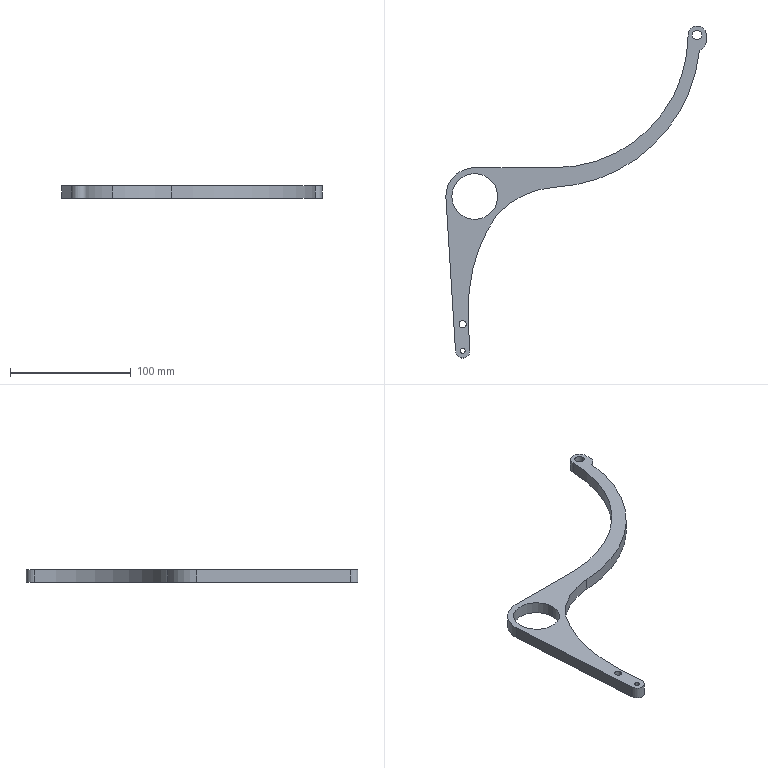Part | SolidWorks | features Extrusion 1 | 1 solid | 21 faces | box 216 x 275.5 x 10 mm | volume 60864 mm3 | cylinder 15 | plane 5 | spline 1 | commonest cylinder face diameters 4 x2 6 x2 7.838 x2 38 x2 12 x1 15 x1
STEP:
#1=CARTESIAN_POINT('',(-3.,22.,10.));
#2=VERTEX_POINT('',#1);
#3=CARTESIAN_POINT('',(3.,22.,10.));
#4=VERTEX_POINT('',#3);
#5=CARTESIAN_POINT('',(0.,22.,10.));
#6=DIRECTION('',(0.,0.,1.));
#7=DIRECTION('',(1.,0.,0.));
#8=AXIS2_PLACEMENT_3D('',#5,#6,#7);
#9=CIRCLE('',#8,3.);
#10=EDGE_CURVE('',#2,#4,#9,.T.);
#11=ORIENTED_EDGE('',*,*,#10,.T.);
#12=CARTESIAN_POINT('',(3.,22.,0.));
#13=VERTEX_POINT('',#12);
#14=CARTESIAN_POINT('',(3.,22.,10.));
#15=DIRECTION('',(0.,0.,-1.));
#16=VECTOR('',#15,1000.);
#17=LINE('',#14,#16);
#18=EDGE_CURVE('',#4,#13,#17,.T.);
#19=ORIENTED_EDGE('',*,*,#18,.T.);
#20=CARTESIAN_POINT('',(-3.,22.,0.));
#21=VERTEX_POINT('',#20);
#22=CARTESIAN_POINT('',(0.,22.,0.));
#23=DIRECTION('',(0.,0.,1.));
#24=DIRECTION('',(1.,0.,0.));
#25=AXIS2_PLACEMENT_3D('',#22,#23,#24);
#26=CIRCLE('',#25,3.);
#27=EDGE_CURVE('',#21,#13,#26,.T.);
#28=ORIENTED_EDGE('',*,*,#27,.F.);
#29=CARTESIAN_POINT('',(-3.,22.,10.));
#30=DIRECTION('',(0.,0.,-1.));
#31=VECTOR('',#30,1000.);
#32=LINE('',#29,#31);
#33=EDGE_CURVE('',#2,#21,#32,.T.);
#34=ORIENTED_EDGE('',*,*,#33,.F.);
#35=EDGE_LOOP('',(#11,#19,#28,#34));
#36=FACE_OUTER_BOUND('',#35,.T.);
#37=CARTESIAN_POINT('',(0.,22.,10.));
#38=DIRECTION('',(0.,0.,-1.));
#39=DIRECTION('',(-1.,0.,0.));
#40=AXIS2_PLACEMENT_3D('',#37,#38,#39);
#41=CYLINDRICAL_SURFACE('',#40,3.);
#42=ADVANCED_FACE('',(#36),#41,.F.);
#43=CARTESIAN_POINT('',(190.581,262.,10.));
#44=VERTEX_POINT('',#43);
#45=CARTESIAN_POINT('',(198.419,262.,10.));
#46=VERTEX_POINT('',#45);
#47=CARTESIAN_POINT('',(194.5,262.,10.));
#48=DIRECTION('',(0.,0.,1.));
#49=DIRECTION('',(1.,0.,0.));
#50=AXIS2_PLACEMENT_3D('',#47,#48,#49);
#51=CIRCLE('',#50,3.919);
#52=EDGE_CURVE('',#44,#46,#51,.T.);
#53=ORIENTED_EDGE('',*,*,#52,.T.);
#54=CARTESIAN_POINT('',(198.419,262.,0.));
#55=VERTEX_POINT('',#54);
#56=CARTESIAN_POINT('',(198.419,262.,10.));
#57=DIRECTION('',(0.,0.,-1.));
#58=VECTOR('',#57,1000.);
#59=LINE('',#56,#58);
#60=EDGE_CURVE('',#46,#55,#59,.T.);
#61=ORIENTED_EDGE('',*,*,#60,.T.);
#62=CARTESIAN_POINT('',(190.581,262.,0.));
#63=VERTEX_POINT('',#62);
#64=CARTESIAN_POINT('',(194.5,262.,0.));
#65=DIRECTION('',(0.,0.,1.));
#66=DIRECTION('',(1.,0.,0.));
#67=AXIS2_PLACEMENT_3D('',#64,#65,#66);
#68=CIRCLE('',#67,3.919);
#69=EDGE_CURVE('',#63,#55,#68,.T.);
#70=ORIENTED_EDGE('',*,*,#69,.F.);
#71=CARTESIAN_POINT('',(190.581,262.,10.));
#72=DIRECTION('',(0.,0.,-1.));
#73=VECTOR('',#72,1000.);
#74=LINE('',#71,#73);
#75=EDGE_CURVE('',#44,#63,#74,.T.);
#76=ORIENTED_EDGE('',*,*,#75,.F.);
#77=EDGE_LOOP('',(#53,#61,#70,#76));
#78=FACE_OUTER_BOUND('',#77,.T.);
#79=CARTESIAN_POINT('',(194.5,262.,10.));
#80=DIRECTION('',(0.,0.,-1.));
#81=DIRECTION('',(-1.,0.,0.));
#82=AXIS2_PLACEMENT_3D('',#79,#80,#81);
#83=CYLINDRICAL_SURFACE('',#82,3.919);
#84=ADVANCED_FACE('',(#78),#83,.F.);
#85=CARTESIAN_POINT('',(-9.,128.,10.));
#86=VERTEX_POINT('',#85);
#87=CARTESIAN_POINT('',(29.,128.,10.));
#88=VERTEX_POINT('',#87);
#89=CARTESIAN_POINT('',(10.,128.,10.));
#90=DIRECTION('',(0.,0.,1.));
#91=DIRECTION('',(1.,0.,0.));
#92=AXIS2_PLACEMENT_3D('',#89,#90,#91);
#93=CIRCLE('',#92,19.);
#94=EDGE_CURVE('',#86,#88,#93,.T.);
#95=ORIENTED_EDGE('',*,*,#94,.T.);
#96=CARTESIAN_POINT('',(29.,128.,0.));
#97=VERTEX_POINT('',#96);
#98=CARTESIAN_POINT('',(29.,128.,10.));
#99=DIRECTION('',(0.,0.,-1.));
#100=VECTOR('',#99,1000.);
#101=LINE('',#98,#100);
#102=EDGE_CURVE('',#88,#97,#101,.T.);
#103=ORIENTED_EDGE('',*,*,#102,.T.);
#104=CARTESIAN_POINT('',(-9.,128.,0.));
#105=VERTEX_POINT('',#104);
#106=CARTESIAN_POINT('',(10.,128.,0.));
#107=DIRECTION('',(0.,0.,1.));
#108=DIRECTION('',(1.,0.,0.));
#109=AXIS2_PLACEMENT_3D('',#106,#107,#108);
#110=CIRCLE('',#109,19.);
#111=EDGE_CURVE('',#105,#97,#110,.T.);
#112=ORIENTED_EDGE('',*,*,#111,.F.);
#113=CARTESIAN_POINT('',(-9.,128.,10.));
#114=DIRECTION('',(0.,0.,-1.));
#115=VECTOR('',#114,1000.);
#116=LINE('',#113,#115);
#117=EDGE_CURVE('',#86,#105,#116,.T.);
#118=ORIENTED_EDGE('',*,*,#117,.F.);
#119=EDGE_LOOP('',(#95,#103,#112,#118));
#120=FACE_OUTER_BOUND('',#119,.T.);
#121=CARTESIAN_POINT('',(10.,128.,10.));
#122=DIRECTION('',(0.,0.,-1.));
#123=DIRECTION('',(-1.,0.,0.));
#124=AXIS2_PLACEMENT_3D('',#121,#122,#123);
#125=CYLINDRICAL_SURFACE('',#124,19.);
#126=ADVANCED_FACE('',(#120),#125,.F.);
#127=CARTESIAN_POINT('',(-2.,0.,10.));
#128=VERTEX_POINT('',#127);
#129=CARTESIAN_POINT('',(2.,0.,10.));
#130=VERTEX_POINT('',#129);
#131=CARTESIAN_POINT('',(0.,0.,10.));
#132=DIRECTION('',(0.,0.,1.));
#133=DIRECTION('',(1.,0.,0.));
#134=AXIS2_PLACEMENT_3D('',#131,#132,#133);
#135=CIRCLE('',#134,2.);
#136=EDGE_CURVE('',#128,#130,#135,.T.);
#137=ORIENTED_EDGE('',*,*,#136,.T.);
#138=CARTESIAN_POINT('',(2.,0.,0.));
#139=VERTEX_POINT('',#138);
#140=CARTESIAN_POINT('',(2.,0.,10.));
#141=DIRECTION('',(0.,0.,-1.));
#142=VECTOR('',#141,1000.);
#143=LINE('',#140,#142);
#144=EDGE_CURVE('',#130,#139,#143,.T.);
#145=ORIENTED_EDGE('',*,*,#144,.T.);
#146=CARTESIAN_POINT('',(-2.,0.,0.));
#147=VERTEX_POINT('',#146);
#148=CARTESIAN_POINT('',(0.,0.,0.));
#149=DIRECTION('',(0.,0.,1.));
#150=DIRECTION('',(1.,0.,0.));
#151=AXIS2_PLACEMENT_3D('',#148,#149,#150);
#152=CIRCLE('',#151,2.);
#153=EDGE_CURVE('',#147,#139,#152,.T.);
#154=ORIENTED_EDGE('',*,*,#153,.F.);
#155=CARTESIAN_POINT('',(-2.,0.,10.));
#156=DIRECTION('',(0.,0.,-1.));
#157=VECTOR('',#156,1000.);
#158=LINE('',#155,#157);
#159=EDGE_CURVE('',#128,#147,#158,.T.);
#160=ORIENTED_EDGE('',*,*,#159,.F.);
#161=EDGE_LOOP('',(#137,#145,#154,#160));
#162=FACE_OUTER_BOUND('',#161,.T.);
#163=CARTESIAN_POINT('',(0.,0.,10.));
#164=DIRECTION('',(0.,0.,-1.));
#165=DIRECTION('',(-1.,0.,0.));
#166=AXIS2_PLACEMENT_3D('',#163,#164,#165);
#167=CYLINDRICAL_SURFACE('',#166,2.);
#168=ADVANCED_FACE('',(#162),#167,.F.);
#169=ORIENTED_EDGE('',*,*,#52,.F.);
#170=CARTESIAN_POINT('',(194.5,262.,10.));
#171=DIRECTION('',(0.,0.,1.));
#172=DIRECTION('',(1.,0.,0.));
#173=AXIS2_PLACEMENT_3D('',#170,#171,#172);
#174=CIRCLE('',#173,3.919);
#175=EDGE_CURVE('',#46,#44,#174,.T.);
#176=ORIENTED_EDGE('',*,*,#175,.F.);
#177=EDGE_LOOP('',(#169,#176));
#178=FACE_BOUND('',#177,.T.);
#179=ORIENTED_EDGE('',*,*,#136,.F.);
#180=CARTESIAN_POINT('',(0.,0.,10.));
#181=DIRECTION('',(0.,0.,1.));
#182=DIRECTION('',(1.,0.,0.));
#183=AXIS2_PLACEMENT_3D('',#180,#181,#182);
#184=CIRCLE('',#183,2.);
#185=EDGE_CURVE('',#130,#128,#184,.T.);
#186=ORIENTED_EDGE('',*,*,#185,.F.);
#187=EDGE_LOOP('',(#179,#186));
#188=FACE_BOUND('',#187,.T.);
#189=CARTESIAN_POINT('',(10.,152.,10.));
#190=VERTEX_POINT('',#189);
#191=CARTESIAN_POINT('',(-14.,128.,10.));
#192=VERTEX_POINT('',#191);
#193=CARTESIAN_POINT('',(10.,128.,10.));
#194=DIRECTION('',(0.,0.,1.));
#195=DIRECTION('',(1.,0.,0.));
#196=AXIS2_PLACEMENT_3D('',#193,#194,#195);
#197=CIRCLE('',#196,24.);
#198=EDGE_CURVE('',#190,#192,#197,.T.);
#199=ORIENTED_EDGE('',*,*,#198,.T.);
#200=CARTESIAN_POINT('',(-6.,0.,10.));
#201=VERTEX_POINT('',#200);
#202=CARTESIAN_POINT('',(-14.,128.,10.));
#203=DIRECTION('',(0.06238,-0.9981,0.));
#204=VECTOR('',#203,1000.);
#205=LINE('',#202,#204);
#206=EDGE_CURVE('',#192,#201,#205,.T.);
#207=ORIENTED_EDGE('',*,*,#206,.T.);
#208=CARTESIAN_POINT('',(6.,0.,10.));
#209=VERTEX_POINT('',#208);
#210=CARTESIAN_POINT('',(0.,0.,10.));
#211=DIRECTION('',(0.,0.,1.));
#212=DIRECTION('',(1.,0.,0.));
#213=AXIS2_PLACEMENT_3D('',#210,#211,#212);
#214=CIRCLE('',#213,6.);
#215=EDGE_CURVE('',#201,#209,#214,.T.);
#216=ORIENTED_EDGE('',*,*,#215,.T.);
#217=CARTESIAN_POINT('',(28.005,112.131,10.));
#218=VERTEX_POINT('',#217);
#219=CARTESIAN_POINT('',(6.,0.,10.));
#220=CARTESIAN_POINT('',(1.589,45.681,10.));
#221=CARTESIAN_POINT('',(5.604,79.643,10.));
#222=CARTESIAN_POINT('',(28.005,112.131,10.));
#223=B_SPLINE_CURVE_WITH_KNOTS('',3,(#219,#220,#221,#222),.UNSPECIFIED.,.F.,.F.,(4,4),(0.,0.7882),.UNSPECIFIED.);
#224=EDGE_CURVE('',#209,#218,#223,.T.);
#225=ORIENTED_EDGE('',*,*,#224,.T.);
#226=CARTESIAN_POINT('',(77.,135.767,10.));
#227=VERTEX_POINT('',#226);
#228=CARTESIAN_POINT('',(80.543,65.825,10.));
#229=DIRECTION('',(0.,0.,-1.));
#230=DIRECTION('',(1.,0.,0.));
#231=AXIS2_PLACEMENT_3D('',#228,#229,#230);
#232=CIRCLE('',#231,70.032);
#233=EDGE_CURVE('',#218,#227,#232,.T.);
#234=ORIENTED_EDGE('',*,*,#233,.T.);
#235=CARTESIAN_POINT('',(196.38,249.495,10.));
#236=VERTEX_POINT('',#235);
#237=CARTESIAN_POINT('',(70.606,262.,10.));
#238=DIRECTION('',(0.,0.,1.));
#239=DIRECTION('',(1.,0.,0.));
#240=AXIS2_PLACEMENT_3D('',#237,#238,#239);
#241=CIRCLE('',#240,126.394);
#242=EDGE_CURVE('',#227,#236,#241,.T.);
#243=ORIENTED_EDGE('',*,*,#242,.T.);
#244=CARTESIAN_POINT('',(202.,257.,10.));
#245=VERTEX_POINT('',#244);
#246=CARTESIAN_POINT('',(194.179,257.,10.));
#247=DIRECTION('',(0.,0.,1.));
#248=DIRECTION('',(1.,0.,0.));
#249=AXIS2_PLACEMENT_3D('',#246,#247,#248);
#250=CIRCLE('',#249,7.821);
#251=EDGE_CURVE('',#236,#245,#250,.T.);
#252=ORIENTED_EDGE('',*,*,#251,.T.);
#253=CARTESIAN_POINT('',(202.,262.,10.));
#254=VERTEX_POINT('',#253);
#255=CARTESIAN_POINT('',(202.,262.,10.));
#256=DIRECTION('',(0.,1.,0.));
#257=VECTOR('',#256,1000.);
#258=LINE('',#255,#257);
#259=EDGE_CURVE('',#245,#254,#258,.T.);
#260=ORIENTED_EDGE('',*,*,#259,.T.);
#261=CARTESIAN_POINT('',(187.,262.,10.));
#262=VERTEX_POINT('',#261);
#263=CARTESIAN_POINT('',(194.5,262.,10.));
#264=DIRECTION('',(0.,0.,1.));
#265=DIRECTION('',(1.,0.,0.));
#266=AXIS2_PLACEMENT_3D('',#263,#264,#265);
#267=CIRCLE('',#266,7.5);
#268=EDGE_CURVE('',#254,#262,#267,.T.);
#269=ORIENTED_EDGE('',*,*,#268,.T.);
#270=CARTESIAN_POINT('',(77.,152.,10.));
#271=VERTEX_POINT('',#270);
#272=CARTESIAN_POINT('',(77.,262.,10.));
#273=DIRECTION('',(0.,0.,-1.));
#274=DIRECTION('',(1.,0.,0.));
#275=AXIS2_PLACEMENT_3D('',#272,#273,#274);
#276=CIRCLE('',#275,110.);
#277=EDGE_CURVE('',#262,#271,#276,.T.);
#278=ORIENTED_EDGE('',*,*,#277,.T.);
#279=CARTESIAN_POINT('',(10.,152.,10.));
#280=DIRECTION('',(-1.,0.,0.));
#281=VECTOR('',#280,1000.);
#282=LINE('',#279,#281);
#283=EDGE_CURVE('',#271,#190,#282,.T.);
#284=ORIENTED_EDGE('',*,*,#283,.T.);
#285=EDGE_LOOP('',(#199,#207,#216,#225,#234,#243,#252,#260,#269,#278,#284));
#286=FACE_OUTER_BOUND('',#285,.T.);
#287=ORIENTED_EDGE('',*,*,#94,.F.);
#288=CARTESIAN_POINT('',(10.,128.,10.));
#289=DIRECTION('',(0.,0.,1.));
#290=DIRECTION('',(1.,0.,0.));
#291=AXIS2_PLACEMENT_3D('',#288,#289,#290);
#292=CIRCLE('',#291,19.);
#293=EDGE_CURVE('',#88,#86,#292,.T.);
#294=ORIENTED_EDGE('',*,*,#293,.F.);
#295=EDGE_LOOP('',(#287,#294));
#296=FACE_BOUND('',#295,.T.);
#297=ORIENTED_EDGE('',*,*,#10,.F.);
#298=CARTESIAN_POINT('',(0.,22.,10.));
#299=DIRECTION('',(0.,0.,1.));
#300=DIRECTION('',(1.,0.,0.));
#301=AXIS2_PLACEMENT_3D('',#298,#299,#300);
#302=CIRCLE('',#301,3.);
#303=EDGE_CURVE('',#4,#2,#302,.T.);
#304=ORIENTED_EDGE('',*,*,#303,.F.);
#305=EDGE_LOOP('',(#297,#304));
#306=FACE_BOUND('',#305,.T.);
#307=CARTESIAN_POINT('',(10.,128.,10.));
#308=DIRECTION('',(0.,0.,1.));
#309=DIRECTION('',(1.,0.,0.));
#310=AXIS2_PLACEMENT_3D('',#307,#308,#309);
#311=PLANE('',#310);
#312=ADVANCED_FACE('',(#178,#188,#286,#296,#306),#311,.T.);
#313=CARTESIAN_POINT('',(10.,152.,0.));
#314=VERTEX_POINT('',#313);
#315=CARTESIAN_POINT('',(-14.,128.,0.));
#316=VERTEX_POINT('',#315);
#317=CARTESIAN_POINT('',(10.,128.,0.));
#318=DIRECTION('',(0.,0.,1.));
#319=DIRECTION('',(1.,0.,0.));
#320=AXIS2_PLACEMENT_3D('',#317,#318,#319);
#321=CIRCLE('',#320,24.);
#322=EDGE_CURVE('',#314,#316,#321,.T.);
#323=ORIENTED_EDGE('',*,*,#322,.F.);
#324=CARTESIAN_POINT('',(77.,152.,0.));
#325=VERTEX_POINT('',#324);
#326=CARTESIAN_POINT('',(10.,152.,0.));
#327=DIRECTION('',(-1.,0.,0.));
#328=VECTOR('',#327,1000.);
#329=LINE('',#326,#328);
#330=EDGE_CURVE('',#325,#314,#329,.T.);
#331=ORIENTED_EDGE('',*,*,#330,.F.);
#332=CARTESIAN_POINT('',(187.,262.,0.));
#333=VERTEX_POINT('',#332);
#334=CARTESIAN_POINT('',(77.,262.,0.));
#335=DIRECTION('',(0.,0.,-1.));
#336=DIRECTION('',(1.,0.,0.));
#337=AXIS2_PLACEMENT_3D('',#334,#335,#336);
#338=CIRCLE('',#337,110.);
#339=EDGE_CURVE('',#333,#325,#338,.T.);
#340=ORIENTED_EDGE('',*,*,#339,.F.);
#341=CARTESIAN_POINT('',(202.,262.,0.));
#342=VERTEX_POINT('',#341);
#343=CARTESIAN_POINT('',(194.5,262.,0.));
#344=DIRECTION('',(0.,0.,1.));
#345=DIRECTION('',(1.,0.,0.));
#346=AXIS2_PLACEMENT_3D('',#343,#344,#345);
#347=CIRCLE('',#346,7.5);
#348=EDGE_CURVE('',#342,#333,#347,.T.);
#349=ORIENTED_EDGE('',*,*,#348,.F.);
#350=CARTESIAN_POINT('',(202.,257.,0.));
#351=VERTEX_POINT('',#350);
#352=CARTESIAN_POINT('',(202.,262.,0.));
#353=DIRECTION('',(0.,1.,0.));
#354=VECTOR('',#353,1000.);
#355=LINE('',#352,#354);
#356=EDGE_CURVE('',#351,#342,#355,.T.);
#357=ORIENTED_EDGE('',*,*,#356,.F.);
#358=CARTESIAN_POINT('',(196.38,249.495,0.));
#359=VERTEX_POINT('',#358);
#360=CARTESIAN_POINT('',(194.179,257.,0.));
#361=DIRECTION('',(0.,0.,1.));
#362=DIRECTION('',(1.,0.,0.));
#363=AXIS2_PLACEMENT_3D('',#360,#361,#362);
#364=CIRCLE('',#363,7.821);
#365=EDGE_CURVE('',#359,#351,#364,.T.);
#366=ORIENTED_EDGE('',*,*,#365,.F.);
#367=CARTESIAN_POINT('',(77.,135.767,0.));
#368=VERTEX_POINT('',#367);
#369=CARTESIAN_POINT('',(70.606,262.,0.));
#370=DIRECTION('',(0.,0.,1.));
#371=DIRECTION('',(1.,0.,0.));
#372=AXIS2_PLACEMENT_3D('',#369,#370,#371);
#373=CIRCLE('',#372,126.394);
#374=EDGE_CURVE('',#368,#359,#373,.T.);
#375=ORIENTED_EDGE('',*,*,#374,.F.);
#376=CARTESIAN_POINT('',(28.005,112.131,0.));
#377=VERTEX_POINT('',#376);
#378=CARTESIAN_POINT('',(80.543,65.825,0.));
#379=DIRECTION('',(0.,0.,-1.));
#380=DIRECTION('',(1.,0.,0.));
#381=AXIS2_PLACEMENT_3D('',#378,#379,#380);
#382=CIRCLE('',#381,70.032);
#383=EDGE_CURVE('',#377,#368,#382,.T.);
#384=ORIENTED_EDGE('',*,*,#383,.F.);
#385=CARTESIAN_POINT('',(6.,0.,0.));
#386=VERTEX_POINT('',#385);
#387=CARTESIAN_POINT('',(6.,0.,0.));
#388=CARTESIAN_POINT('',(1.589,45.681,0.));
#389=CARTESIAN_POINT('',(5.604,79.643,0.));
#390=CARTESIAN_POINT('',(28.005,112.131,0.));
#391=B_SPLINE_CURVE_WITH_KNOTS('',3,(#387,#388,#389,#390),.UNSPECIFIED.,.F.,.F.,(4,4),(0.,0.7882),.UNSPECIFIED.);
#392=EDGE_CURVE('',#386,#377,#391,.T.);
#393=ORIENTED_EDGE('',*,*,#392,.F.);
#394=CARTESIAN_POINT('',(-6.,0.,0.));
#395=VERTEX_POINT('',#394);
#396=CARTESIAN_POINT('',(0.,0.,0.));
#397=DIRECTION('',(0.,0.,1.));
#398=DIRECTION('',(1.,0.,0.));
#399=AXIS2_PLACEMENT_3D('',#396,#397,#398);
#400=CIRCLE('',#399,6.);
#401=EDGE_CURVE('',#395,#386,#400,.T.);
#402=ORIENTED_EDGE('',*,*,#401,.F.);
#403=CARTESIAN_POINT('',(-14.,128.,0.));
#404=DIRECTION('',(0.06238,-0.9981,0.));
#405=VECTOR('',#404,1000.);
#406=LINE('',#403,#405);
#407=EDGE_CURVE('',#316,#395,#406,.T.);
#408=ORIENTED_EDGE('',*,*,#407,.F.);
#409=EDGE_LOOP('',(#323,#331,#340,#349,#357,#366,#375,#384,#393,#402,#408));
#410=FACE_OUTER_BOUND('',#409,.T.);
#411=ORIENTED_EDGE('',*,*,#153,.T.);
#412=CARTESIAN_POINT('',(0.,0.,0.));
#413=DIRECTION('',(0.,0.,1.));
#414=DIRECTION('',(1.,0.,0.));
#415=AXIS2_PLACEMENT_3D('',#412,#413,#414);
#416=CIRCLE('',#415,2.);
#417=EDGE_CURVE('',#139,#147,#416,.T.);
#418=ORIENTED_EDGE('',*,*,#417,.T.);
#419=EDGE_LOOP('',(#411,#418));
#420=FACE_BOUND('',#419,.T.);
#421=ORIENTED_EDGE('',*,*,#111,.T.);
#422=CARTESIAN_POINT('',(10.,128.,0.));
#423=DIRECTION('',(0.,0.,1.));
#424=DIRECTION('',(1.,0.,0.));
#425=AXIS2_PLACEMENT_3D('',#422,#423,#424);
#426=CIRCLE('',#425,19.);
#427=EDGE_CURVE('',#97,#105,#426,.T.);
#428=ORIENTED_EDGE('',*,*,#427,.T.);
#429=EDGE_LOOP('',(#421,#428));
#430=FACE_BOUND('',#429,.T.);
#431=ORIENTED_EDGE('',*,*,#69,.T.);
#432=CARTESIAN_POINT('',(194.5,262.,0.));
#433=DIRECTION('',(0.,0.,1.));
#434=DIRECTION('',(1.,0.,0.));
#435=AXIS2_PLACEMENT_3D('',#432,#433,#434);
#436=CIRCLE('',#435,3.919);
#437=EDGE_CURVE('',#55,#63,#436,.T.);
#438=ORIENTED_EDGE('',*,*,#437,.T.);
#439=EDGE_LOOP('',(#431,#438));
#440=FACE_BOUND('',#439,.T.);
#441=ORIENTED_EDGE('',*,*,#27,.T.);
#442=CARTESIAN_POINT('',(0.,22.,0.));
#443=DIRECTION('',(0.,0.,1.));
#444=DIRECTION('',(1.,0.,0.));
#445=AXIS2_PLACEMENT_3D('',#442,#443,#444);
#446=CIRCLE('',#445,3.);
#447=EDGE_CURVE('',#13,#21,#446,.T.);
#448=ORIENTED_EDGE('',*,*,#447,.T.);
#449=EDGE_LOOP('',(#441,#448));
#450=FACE_BOUND('',#449,.T.);
#451=CARTESIAN_POINT('',(10.,128.,0.));
#452=DIRECTION('',(0.,0.,1.));
#453=DIRECTION('',(1.,0.,0.));
#454=AXIS2_PLACEMENT_3D('',#451,#452,#453);
#455=PLANE('',#454);
#456=ADVANCED_FACE('',(#410,#420,#430,#440,#450),#455,.F.);
#457=ORIENTED_EDGE('',*,*,#322,.T.);
#458=CARTESIAN_POINT('',(-14.,128.,10.));
#459=DIRECTION('',(0.,0.,-1.));
#460=VECTOR('',#459,1000.);
#461=LINE('',#458,#460);
#462=EDGE_CURVE('',#192,#316,#461,.T.);
#463=ORIENTED_EDGE('',*,*,#462,.F.);
#464=ORIENTED_EDGE('',*,*,#198,.F.);
#465=CARTESIAN_POINT('',(10.,152.,10.));
#466=DIRECTION('',(0.,0.,-1.));
#467=VECTOR('',#466,1000.);
#468=LINE('',#465,#467);
#469=EDGE_CURVE('',#190,#314,#468,.T.);
#470=ORIENTED_EDGE('',*,*,#469,.T.);
#471=EDGE_LOOP('',(#457,#463,#464,#470));
#472=FACE_OUTER_BOUND('',#471,.T.);
#473=CARTESIAN_POINT('',(10.,128.,10.));
#474=DIRECTION('',(0.,0.,-1.));
#475=DIRECTION('',(-1.,0.,0.));
#476=AXIS2_PLACEMENT_3D('',#473,#474,#475);
#477=CYLINDRICAL_SURFACE('',#476,24.);
#478=ADVANCED_FACE('',(#472),#477,.T.);
#479=ORIENTED_EDGE('',*,*,#407,.T.);
#480=CARTESIAN_POINT('',(-6.,0.,10.));
#481=DIRECTION('',(0.,0.,-1.));
#482=VECTOR('',#481,1000.);
#483=LINE('',#480,#482);
#484=EDGE_CURVE('',#201,#395,#483,.T.);
#485=ORIENTED_EDGE('',*,*,#484,.F.);
#486=ORIENTED_EDGE('',*,*,#206,.F.);
#487=ORIENTED_EDGE('',*,*,#462,.T.);
#488=EDGE_LOOP('',(#479,#485,#486,#487));
#489=FACE_OUTER_BOUND('',#488,.T.);
#490=CARTESIAN_POINT('',(-14.,128.,10.));
#491=DIRECTION('',(0.9981,0.06238,0.));
#492=DIRECTION('',(-0.06238,0.9981,0.));
#493=AXIS2_PLACEMENT_3D('',#490,#491,#492);
#494=PLANE('',#493);
#495=ADVANCED_FACE('',(#489),#494,.F.);
#496=ORIENTED_EDGE('',*,*,#401,.T.);
#497=CARTESIAN_POINT('',(6.,0.,10.));
#498=DIRECTION('',(0.,0.,-1.));
#499=VECTOR('',#498,1000.);
#500=LINE('',#497,#499);
#501=EDGE_CURVE('',#209,#386,#500,.T.);
#502=ORIENTED_EDGE('',*,*,#501,.F.);
#503=ORIENTED_EDGE('',*,*,#215,.F.);
#504=ORIENTED_EDGE('',*,*,#484,.T.);
#505=EDGE_LOOP('',(#496,#502,#503,#504));
#506=FACE_OUTER_BOUND('',#505,.T.);
#507=CARTESIAN_POINT('',(0.,0.,10.));
#508=DIRECTION('',(0.,0.,-1.));
#509=DIRECTION('',(-1.,0.,0.));
#510=AXIS2_PLACEMENT_3D('',#507,#508,#509);
#511=CYLINDRICAL_SURFACE('',#510,6.);
#512=ADVANCED_FACE('',(#506),#511,.T.);
#513=ORIENTED_EDGE('',*,*,#392,.T.);
#514=CARTESIAN_POINT('',(28.005,112.131,10.));
#515=DIRECTION('',(0.,0.,-1.));
#516=VECTOR('',#515,1000.);
#517=LINE('',#514,#516);
#518=EDGE_CURVE('',#218,#377,#517,.T.);
#519=ORIENTED_EDGE('',*,*,#518,.F.);
#520=ORIENTED_EDGE('',*,*,#224,.F.);
#521=ORIENTED_EDGE('',*,*,#501,.T.);
#522=EDGE_LOOP('',(#513,#519,#520,#521));
#523=FACE_OUTER_BOUND('',#522,.T.);
#524=CARTESIAN_POINT('',(6.,0.,10.));
#525=CARTESIAN_POINT('',(6.,0.,0.));
#526=CARTESIAN_POINT('',(1.589,45.681,10.));
#527=CARTESIAN_POINT('',(1.589,45.681,0.));
#528=CARTESIAN_POINT('',(5.604,79.643,10.));
#529=CARTESIAN_POINT('',(5.604,79.643,0.));
#530=CARTESIAN_POINT('',(28.005,112.131,10.));
#531=CARTESIAN_POINT('',(28.005,112.131,0.));
#532=B_SPLINE_SURFACE_WITH_KNOTS('',3,1,((#524,#525),(#526,#527),(#528,#529),(#530,#531)),.UNSPECIFIED.,.F.,.F.,.F.,(4,4),(2,2),(0.,0.7882),(0.,1.),.UNSPECIFIED.);
#533=ADVANCED_FACE('',(#523),#532,.F.);
#534=ORIENTED_EDGE('',*,*,#383,.T.);
#535=CARTESIAN_POINT('',(77.,135.767,10.));
#536=DIRECTION('',(0.,0.,-1.));
#537=VECTOR('',#536,1000.);
#538=LINE('',#535,#537);
#539=EDGE_CURVE('',#227,#368,#538,.T.);
#540=ORIENTED_EDGE('',*,*,#539,.F.);
#541=ORIENTED_EDGE('',*,*,#233,.F.);
#542=ORIENTED_EDGE('',*,*,#518,.T.);
#543=EDGE_LOOP('',(#534,#540,#541,#542));
#544=FACE_OUTER_BOUND('',#543,.T.);
#545=CARTESIAN_POINT('',(80.543,65.825,10.));
#546=DIRECTION('',(0.,0.,-1.));
#547=DIRECTION('',(-1.,0.,0.));
#548=AXIS2_PLACEMENT_3D('',#545,#546,#547);
#549=CYLINDRICAL_SURFACE('',#548,70.032);
#550=ADVANCED_FACE('',(#544),#549,.F.);
#551=ORIENTED_EDGE('',*,*,#374,.T.);
#552=CARTESIAN_POINT('',(196.38,249.495,10.));
#553=DIRECTION('',(0.,0.,-1.));
#554=VECTOR('',#553,1000.);
#555=LINE('',#552,#554);
#556=EDGE_CURVE('',#236,#359,#555,.T.);
#557=ORIENTED_EDGE('',*,*,#556,.F.);
#558=ORIENTED_EDGE('',*,*,#242,.F.);
#559=ORIENTED_EDGE('',*,*,#539,.T.);
#560=EDGE_LOOP('',(#551,#557,#558,#559));
#561=FACE_OUTER_BOUND('',#560,.T.);
#562=CARTESIAN_POINT('',(70.606,262.,10.));
#563=DIRECTION('',(0.,0.,-1.));
#564=DIRECTION('',(-1.,0.,0.));
#565=AXIS2_PLACEMENT_3D('',#562,#563,#564);
#566=CYLINDRICAL_SURFACE('',#565,126.394);
#567=ADVANCED_FACE('',(#561),#566,.T.);
#568=ORIENTED_EDGE('',*,*,#365,.T.);
#569=CARTESIAN_POINT('',(202.,257.,10.));
#570=DIRECTION('',(0.,0.,-1.));
#571=VECTOR('',#570,1000.);
#572=LINE('',#569,#571);
#573=EDGE_CURVE('',#245,#351,#572,.T.);
#574=ORIENTED_EDGE('',*,*,#573,.F.);
#575=ORIENTED_EDGE('',*,*,#251,.F.);
#576=ORIENTED_EDGE('',*,*,#556,.T.);
#577=EDGE_LOOP('',(#568,#574,#575,#576));
#578=FACE_OUTER_BOUND('',#577,.T.);
#579=CARTESIAN_POINT('',(194.179,257.,10.));
#580=DIRECTION('',(0.,0.,-1.));
#581=DIRECTION('',(-1.,0.,0.));
#582=AXIS2_PLACEMENT_3D('',#579,#580,#581);
#583=CYLINDRICAL_SURFACE('',#582,7.821);
#584=ADVANCED_FACE('',(#578),#583,.T.);
#585=ORIENTED_EDGE('',*,*,#356,.T.);
#586=CARTESIAN_POINT('',(202.,262.,10.));
#587=DIRECTION('',(0.,0.,-1.));
#588=VECTOR('',#587,1000.);
#589=LINE('',#586,#588);
#590=EDGE_CURVE('',#254,#342,#589,.T.);
#591=ORIENTED_EDGE('',*,*,#590,.F.);
#592=ORIENTED_EDGE('',*,*,#259,.F.);
#593=ORIENTED_EDGE('',*,*,#573,.T.);
#594=EDGE_LOOP('',(#585,#591,#592,#593));
#595=FACE_OUTER_BOUND('',#594,.T.);
#596=CARTESIAN_POINT('',(202.,262.,10.));
#597=DIRECTION('',(-1.,0.,0.));
#598=DIRECTION('',(0.,0.,1.));
#599=AXIS2_PLACEMENT_3D('',#596,#597,#598);
#600=PLANE('',#599);
#601=ADVANCED_FACE('',(#595),#600,.F.);
#602=ORIENTED_EDGE('',*,*,#348,.T.);
#603=CARTESIAN_POINT('',(187.,262.,10.));
#604=DIRECTION('',(0.,0.,-1.));
#605=VECTOR('',#604,1000.);
#606=LINE('',#603,#605);
#607=EDGE_CURVE('',#262,#333,#606,.T.);
#608=ORIENTED_EDGE('',*,*,#607,.F.);
#609=ORIENTED_EDGE('',*,*,#268,.F.);
#610=ORIENTED_EDGE('',*,*,#590,.T.);
#611=EDGE_LOOP('',(#602,#608,#609,#610));
#612=FACE_OUTER_BOUND('',#611,.T.);
#613=CARTESIAN_POINT('',(194.5,262.,10.));
#614=DIRECTION('',(0.,0.,-1.));
#615=DIRECTION('',(-1.,0.,0.));
#616=AXIS2_PLACEMENT_3D('',#613,#614,#615);
#617=CYLINDRICAL_SURFACE('',#616,7.5);
#618=ADVANCED_FACE('',(#612),#617,.T.);
#619=ORIENTED_EDGE('',*,*,#339,.T.);
#620=CARTESIAN_POINT('',(77.,152.,10.));
#621=DIRECTION('',(0.,0.,-1.));
#622=VECTOR('',#621,1000.);
#623=LINE('',#620,#622);
#624=EDGE_CURVE('',#271,#325,#623,.T.);
#625=ORIENTED_EDGE('',*,*,#624,.F.);
#626=ORIENTED_EDGE('',*,*,#277,.F.);
#627=ORIENTED_EDGE('',*,*,#607,.T.);
#628=EDGE_LOOP('',(#619,#625,#626,#627));
#629=FACE_OUTER_BOUND('',#628,.T.);
#630=CARTESIAN_POINT('',(77.,262.,10.));
#631=DIRECTION('',(0.,0.,-1.));
#632=DIRECTION('',(-1.,0.,0.));
#633=AXIS2_PLACEMENT_3D('',#630,#631,#632);
#634=CYLINDRICAL_SURFACE('',#633,110.);
#635=ADVANCED_FACE('',(#629),#634,.F.);
#636=ORIENTED_EDGE('',*,*,#330,.T.);
#637=ORIENTED_EDGE('',*,*,#469,.F.);
#638=ORIENTED_EDGE('',*,*,#283,.F.);
#639=ORIENTED_EDGE('',*,*,#624,.T.);
#640=EDGE_LOOP('',(#636,#637,#638,#639));
#641=FACE_OUTER_BOUND('',#640,.T.);
#642=CARTESIAN_POINT('',(10.,152.,10.));
#643=DIRECTION('',(0.,-1.,0.));
#644=DIRECTION('',(1.,0.,0.));
#645=AXIS2_PLACEMENT_3D('',#642,#643,#644);
#646=PLANE('',#645);
#647=ADVANCED_FACE('',(#641),#646,.F.);
#648=ORIENTED_EDGE('',*,*,#144,.F.);
#649=ORIENTED_EDGE('',*,*,#185,.T.);
#650=ORIENTED_EDGE('',*,*,#159,.T.);
#651=ORIENTED_EDGE('',*,*,#417,.F.);
#652=EDGE_LOOP('',(#648,#649,#650,#651));
#653=FACE_OUTER_BOUND('',#652,.T.);
#654=CARTESIAN_POINT('',(0.,0.,10.));
#655=DIRECTION('',(0.,0.,-1.));
#656=DIRECTION('',(-1.,0.,0.));
#657=AXIS2_PLACEMENT_3D('',#654,#655,#656);
#658=CYLINDRICAL_SURFACE('',#657,2.);
#659=ADVANCED_FACE('',(#653),#658,.F.);
#660=ORIENTED_EDGE('',*,*,#102,.F.);
#661=ORIENTED_EDGE('',*,*,#293,.T.);
#662=ORIENTED_EDGE('',*,*,#117,.T.);
#663=ORIENTED_EDGE('',*,*,#427,.F.);
#664=EDGE_LOOP('',(#660,#661,#662,#663));
#665=FACE_OUTER_BOUND('',#664,.T.);
#666=CARTESIAN_POINT('',(10.,128.,10.));
#667=DIRECTION('',(0.,0.,-1.));
#668=DIRECTION('',(-1.,0.,0.));
#669=AXIS2_PLACEMENT_3D('',#666,#667,#668);
#670=CYLINDRICAL_SURFACE('',#669,19.);
#671=ADVANCED_FACE('',(#665),#670,.F.);
#672=ORIENTED_EDGE('',*,*,#60,.F.);
#673=ORIENTED_EDGE('',*,*,#175,.T.);
#674=ORIENTED_EDGE('',*,*,#75,.T.);
#675=ORIENTED_EDGE('',*,*,#437,.F.);
#676=EDGE_LOOP('',(#672,#673,#674,#675));
#677=FACE_OUTER_BOUND('',#676,.T.);
#678=CARTESIAN_POINT('',(194.5,262.,10.));
#679=DIRECTION('',(0.,0.,-1.));
#680=DIRECTION('',(-1.,0.,0.));
#681=AXIS2_PLACEMENT_3D('',#678,#679,#680);
#682=CYLINDRICAL_SURFACE('',#681,3.919);
#683=ADVANCED_FACE('',(#677),#682,.F.);
#684=ORIENTED_EDGE('',*,*,#18,.F.);
#685=ORIENTED_EDGE('',*,*,#303,.T.);
#686=ORIENTED_EDGE('',*,*,#33,.T.);
#687=ORIENTED_EDGE('',*,*,#447,.F.);
#688=EDGE_LOOP('',(#684,#685,#686,#687));
#689=FACE_OUTER_BOUND('',#688,.T.);
#690=CARTESIAN_POINT('',(0.,22.,10.));
#691=DIRECTION('',(0.,0.,-1.));
#692=DIRECTION('',(-1.,0.,0.));
#693=AXIS2_PLACEMENT_3D('',#690,#691,#692);
#694=CYLINDRICAL_SURFACE('',#693,3.);
#695=ADVANCED_FACE('',(#689),#694,.F.);
#696=CLOSED_SHELL('',(#42,#84,#126,#168,#312,#456,#478,#495,#512,#533,#550,#567,#584,#601,#618,#635,#647,#659,#671,#683,#695));
#697=MANIFOLD_SOLID_BREP('',#696);
#698=CARTESIAN_POINT('',(0.,0.,0.));
#699=DIRECTION('',(0.,0.,1.));
#700=DIRECTION('',(1.,0.,0.));
#701=AXIS2_PLACEMENT_3D('',#698,#699,#700);
#702=(LENGTH_UNIT()NAMED_UNIT(*)SI_UNIT(.MILLI.,.METRE.));
#703=UNCERTAINTY_MEASURE_WITH_UNIT(LENGTH_MEASURE(0.00001),#702,'','');
#704=(NAMED_UNIT(*)PLANE_ANGLE_UNIT()SI_UNIT($,.RADIAN.));
#705=(NAMED_UNIT(*)SI_UNIT($,.STERADIAN.)SOLID_ANGLE_UNIT());
#706=(GEOMETRIC_REPRESENTATION_CONTEXT(3)GLOBAL_UNCERTAINTY_ASSIGNED_CONTEXT((#703))GLOBAL_UNIT_ASSIGNED_CONTEXT((#702,#704,#705))REPRESENTATION_CONTEXT('',''));
#707=ADVANCED_BREP_SHAPE_REPRESENTATION('',(#697,#701),#706);